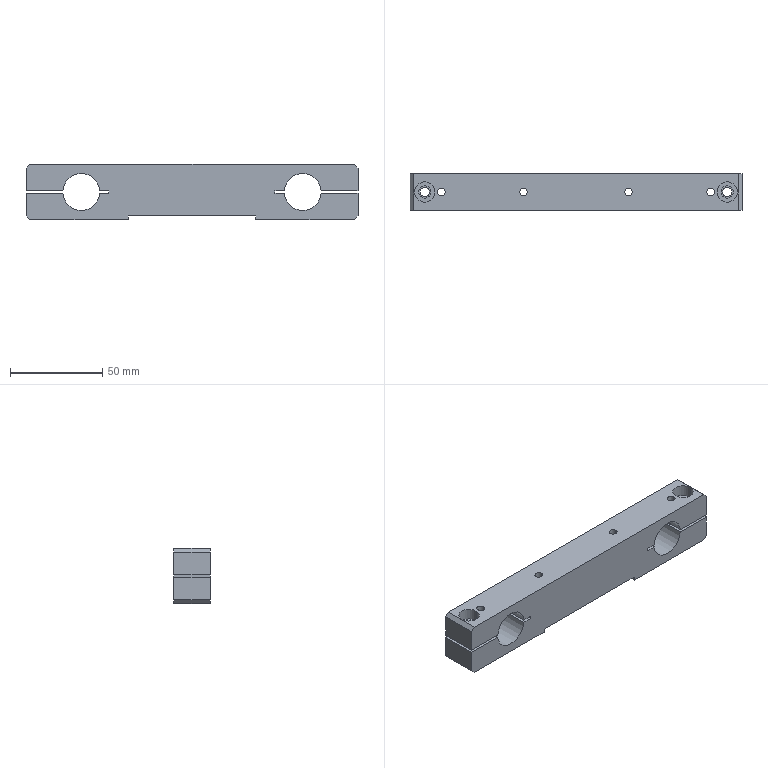Part | STEP file | 11-FG-S01611 | 1 solid | 58 faces | box 180 x 20 x 30 mm | volume 87134 mm3 | cylinder 30 | plane 28 | commonest cylinder face diameters 4.2 x12 20 x6 5 x4 6.6 x4 11 x4